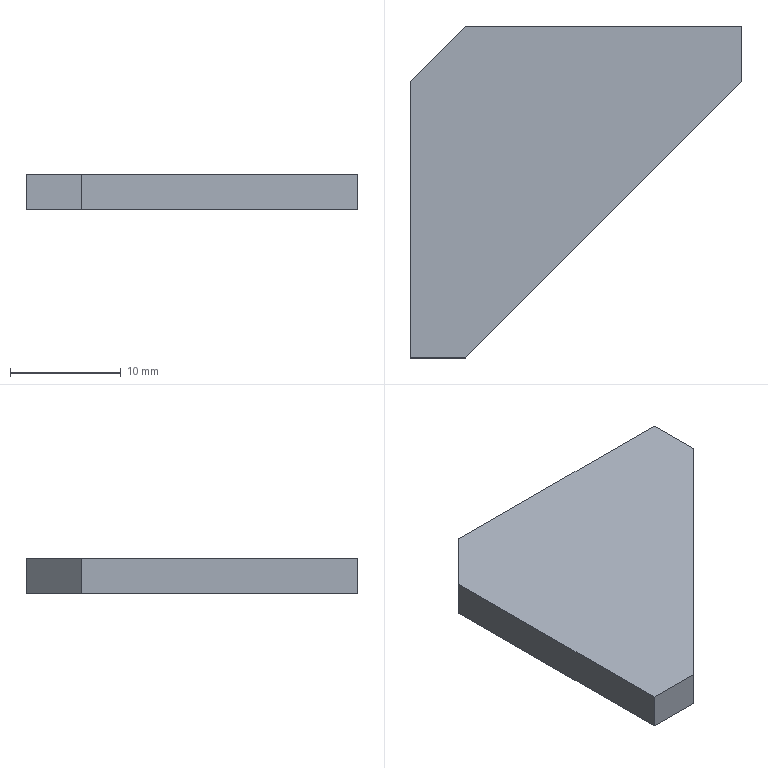Part | SolidWorks | features FlatPattern 1, SMBaseFlange 1, SheetMetal 1 | 1 solid | 8 faces | box 30 x 30 x 3.2 mm | volume 1840 mm3 | plane 8
STEP:
#1=CARTESIAN_POINT('',(268.2,-169.019,0.));
#2=VERTEX_POINT('',#1);
#3=CARTESIAN_POINT('',(243.2,-169.019,0.));
#4=VERTEX_POINT('',#3);
#5=CARTESIAN_POINT('',(243.2,-169.019,0.));
#6=DIRECTION('',(-1.,0.,0.));
#7=VECTOR('',#6,1000.);
#8=LINE('',#5,#7);
#9=EDGE_CURVE('',#2,#4,#8,.T.);
#10=ORIENTED_EDGE('',*,*,#9,.F.);
#11=CARTESIAN_POINT('',(268.2,-169.019,-3.2));
#12=VERTEX_POINT('',#11);
#13=CARTESIAN_POINT('',(268.2,-169.019,-3.2));
#14=DIRECTION('',(0.,0.,1.));
#15=VECTOR('',#14,1000.);
#16=LINE('',#13,#15);
#17=EDGE_CURVE('',#12,#2,#16,.T.);
#18=ORIENTED_EDGE('',*,*,#17,.F.);
#19=CARTESIAN_POINT('',(243.2,-169.019,-3.2));
#20=VERTEX_POINT('',#19);
#21=CARTESIAN_POINT('',(243.2,-169.019,-3.2));
#22=DIRECTION('',(-1.,0.,0.));
#23=VECTOR('',#22,1000.);
#24=LINE('',#21,#23);
#25=EDGE_CURVE('',#12,#20,#24,.T.);
#26=ORIENTED_EDGE('',*,*,#25,.T.);
#27=CARTESIAN_POINT('',(243.2,-169.019,-3.2));
#28=DIRECTION('',(0.,0.,1.));
#29=VECTOR('',#28,1000.);
#30=LINE('',#27,#29);
#31=EDGE_CURVE('',#20,#4,#30,.T.);
#32=ORIENTED_EDGE('',*,*,#31,.T.);
#33=EDGE_LOOP('',(#10,#18,#26,#32));
#34=FACE_OUTER_BOUND('',#33,.T.);
#35=CARTESIAN_POINT('',(243.2,-169.019,-3.2));
#36=DIRECTION('',(0.,1.,0.));
#37=DIRECTION('',(0.,0.,1.));
#38=AXIS2_PLACEMENT_3D('',#35,#36,#37);
#39=PLANE('',#38);
#40=ADVANCED_FACE('',(#34),#39,.T.);
#41=CARTESIAN_POINT('',(268.2,-174.019,0.));
#42=VERTEX_POINT('',#41);
#43=CARTESIAN_POINT('',(268.2,-169.019,0.));
#44=DIRECTION('',(0.,1.,0.));
#45=VECTOR('',#44,1000.);
#46=LINE('',#43,#45);
#47=EDGE_CURVE('',#42,#2,#46,.T.);
#48=ORIENTED_EDGE('',*,*,#47,.F.);
#49=CARTESIAN_POINT('',(268.2,-174.019,-3.2));
#50=VERTEX_POINT('',#49);
#51=CARTESIAN_POINT('',(268.2,-174.019,-3.2));
#52=DIRECTION('',(0.,0.,1.));
#53=VECTOR('',#52,1000.);
#54=LINE('',#51,#53);
#55=EDGE_CURVE('',#50,#42,#54,.T.);
#56=ORIENTED_EDGE('',*,*,#55,.F.);
#57=CARTESIAN_POINT('',(268.2,-169.019,-3.2));
#58=DIRECTION('',(0.,1.,0.));
#59=VECTOR('',#58,1000.);
#60=LINE('',#57,#59);
#61=EDGE_CURVE('',#50,#12,#60,.T.);
#62=ORIENTED_EDGE('',*,*,#61,.T.);
#63=ORIENTED_EDGE('',*,*,#17,.T.);
#64=EDGE_LOOP('',(#48,#56,#62,#63));
#65=FACE_OUTER_BOUND('',#64,.T.);
#66=CARTESIAN_POINT('',(268.2,-169.019,-3.2));
#67=DIRECTION('',(1.,0.,0.));
#68=DIRECTION('',(0.,0.,-1.));
#69=AXIS2_PLACEMENT_3D('',#66,#67,#68);
#70=PLANE('',#69);
#71=ADVANCED_FACE('',(#65),#70,.T.);
#72=CARTESIAN_POINT('',(243.2,-199.019,0.));
#73=VERTEX_POINT('',#72);
#74=CARTESIAN_POINT('',(268.2,-174.019,0.));
#75=DIRECTION('',(0.7071,0.7071,0.));
#76=VECTOR('',#75,1000.);
#77=LINE('',#74,#76);
#78=EDGE_CURVE('',#73,#42,#77,.T.);
#79=ORIENTED_EDGE('',*,*,#78,.F.);
#80=CARTESIAN_POINT('',(243.2,-199.019,-3.2));
#81=VERTEX_POINT('',#80);
#82=CARTESIAN_POINT('',(243.2,-199.019,-3.2));
#83=DIRECTION('',(0.,0.,1.));
#84=VECTOR('',#83,1000.);
#85=LINE('',#82,#84);
#86=EDGE_CURVE('',#81,#73,#85,.T.);
#87=ORIENTED_EDGE('',*,*,#86,.F.);
#88=CARTESIAN_POINT('',(268.2,-174.019,-3.2));
#89=DIRECTION('',(0.7071,0.7071,0.));
#90=VECTOR('',#89,1000.);
#91=LINE('',#88,#90);
#92=EDGE_CURVE('',#81,#50,#91,.T.);
#93=ORIENTED_EDGE('',*,*,#92,.T.);
#94=ORIENTED_EDGE('',*,*,#55,.T.);
#95=EDGE_LOOP('',(#79,#87,#93,#94));
#96=FACE_OUTER_BOUND('',#95,.T.);
#97=CARTESIAN_POINT('',(268.2,-174.019,-3.2));
#98=DIRECTION('',(0.7071,-0.7071,0.));
#99=DIRECTION('',(0.7071,0.7071,0.));
#100=AXIS2_PLACEMENT_3D('',#97,#98,#99);
#101=PLANE('',#100);
#102=ADVANCED_FACE('',(#96),#101,.T.);
#103=CARTESIAN_POINT('',(238.2,-199.019,0.));
#104=VERTEX_POINT('',#103);
#105=CARTESIAN_POINT('',(243.2,-199.019,0.));
#106=DIRECTION('',(1.,0.,0.));
#107=VECTOR('',#106,1000.);
#108=LINE('',#105,#107);
#109=EDGE_CURVE('',#104,#73,#108,.T.);
#110=ORIENTED_EDGE('',*,*,#109,.F.);
#111=CARTESIAN_POINT('',(238.2,-199.019,-3.2));
#112=VERTEX_POINT('',#111);
#113=CARTESIAN_POINT('',(238.2,-199.019,-3.2));
#114=DIRECTION('',(0.,0.,1.));
#115=VECTOR('',#114,1000.);
#116=LINE('',#113,#115);
#117=EDGE_CURVE('',#112,#104,#116,.T.);
#118=ORIENTED_EDGE('',*,*,#117,.F.);
#119=CARTESIAN_POINT('',(243.2,-199.019,-3.2));
#120=DIRECTION('',(1.,0.,0.));
#121=VECTOR('',#120,1000.);
#122=LINE('',#119,#121);
#123=EDGE_CURVE('',#112,#81,#122,.T.);
#124=ORIENTED_EDGE('',*,*,#123,.T.);
#125=ORIENTED_EDGE('',*,*,#86,.T.);
#126=EDGE_LOOP('',(#110,#118,#124,#125));
#127=FACE_OUTER_BOUND('',#126,.T.);
#128=CARTESIAN_POINT('',(243.2,-199.019,-3.2));
#129=DIRECTION('',(0.,-1.,0.));
#130=DIRECTION('',(0.,0.,-1.));
#131=AXIS2_PLACEMENT_3D('',#128,#129,#130);
#132=PLANE('',#131);
#133=ADVANCED_FACE('',(#127),#132,.T.);
#134=CARTESIAN_POINT('',(238.2,-174.019,0.));
#135=VERTEX_POINT('',#134);
#136=CARTESIAN_POINT('',(238.2,-199.019,0.));
#137=DIRECTION('',(0.,-1.,0.));
#138=VECTOR('',#137,1000.);
#139=LINE('',#136,#138);
#140=EDGE_CURVE('',#135,#104,#139,.T.);
#141=ORIENTED_EDGE('',*,*,#140,.F.);
#142=CARTESIAN_POINT('',(238.2,-174.019,-3.2));
#143=VERTEX_POINT('',#142);
#144=CARTESIAN_POINT('',(238.2,-174.019,-3.2));
#145=DIRECTION('',(0.,0.,1.));
#146=VECTOR('',#145,1000.);
#147=LINE('',#144,#146);
#148=EDGE_CURVE('',#143,#135,#147,.T.);
#149=ORIENTED_EDGE('',*,*,#148,.F.);
#150=CARTESIAN_POINT('',(238.2,-199.019,-3.2));
#151=DIRECTION('',(0.,-1.,0.));
#152=VECTOR('',#151,1000.);
#153=LINE('',#150,#152);
#154=EDGE_CURVE('',#143,#112,#153,.T.);
#155=ORIENTED_EDGE('',*,*,#154,.T.);
#156=ORIENTED_EDGE('',*,*,#117,.T.);
#157=EDGE_LOOP('',(#141,#149,#155,#156));
#158=FACE_OUTER_BOUND('',#157,.T.);
#159=CARTESIAN_POINT('',(238.2,-199.019,-3.2));
#160=DIRECTION('',(-1.,0.,0.));
#161=DIRECTION('',(0.,0.,1.));
#162=AXIS2_PLACEMENT_3D('',#159,#160,#161);
#163=PLANE('',#162);
#164=ADVANCED_FACE('',(#158),#163,.T.);
#165=CARTESIAN_POINT('',(238.2,-174.019,0.));
#166=DIRECTION('',(-0.7071,-0.7071,0.));
#167=VECTOR('',#166,1000.);
#168=LINE('',#165,#167);
#169=EDGE_CURVE('',#4,#135,#168,.T.);
#170=ORIENTED_EDGE('',*,*,#169,.F.);
#171=ORIENTED_EDGE('',*,*,#31,.F.);
#172=CARTESIAN_POINT('',(238.2,-174.019,-3.2));
#173=DIRECTION('',(-0.7071,-0.7071,0.));
#174=VECTOR('',#173,1000.);
#175=LINE('',#172,#174);
#176=EDGE_CURVE('',#20,#143,#175,.T.);
#177=ORIENTED_EDGE('',*,*,#176,.T.);
#178=ORIENTED_EDGE('',*,*,#148,.T.);
#179=EDGE_LOOP('',(#170,#171,#177,#178));
#180=FACE_OUTER_BOUND('',#179,.T.);
#181=CARTESIAN_POINT('',(238.2,-174.019,-3.2));
#182=DIRECTION('',(-0.7071,0.7071,0.));
#183=DIRECTION('',(-0.7071,-0.7071,0.));
#184=AXIS2_PLACEMENT_3D('',#181,#182,#183);
#185=PLANE('',#184);
#186=ADVANCED_FACE('',(#180),#185,.T.);
#187=ORIENTED_EDGE('',*,*,#25,.F.);
#188=ORIENTED_EDGE('',*,*,#61,.F.);
#189=ORIENTED_EDGE('',*,*,#92,.F.);
#190=ORIENTED_EDGE('',*,*,#123,.F.);
#191=ORIENTED_EDGE('',*,*,#154,.F.);
#192=ORIENTED_EDGE('',*,*,#176,.F.);
#193=EDGE_LOOP('',(#187,#188,#189,#190,#191,#192));
#194=FACE_OUTER_BOUND('',#193,.T.);
#195=CARTESIAN_POINT('',(0.,0.,-3.2));
#196=DIRECTION('',(0.,0.,-1.));
#197=DIRECTION('',(-1.,0.,0.));
#198=AXIS2_PLACEMENT_3D('',#195,#196,#197);
#199=PLANE('',#198);
#200=ADVANCED_FACE('',(#194),#199,.T.);
#201=ORIENTED_EDGE('',*,*,#9,.T.);
#202=ORIENTED_EDGE('',*,*,#169,.T.);
#203=ORIENTED_EDGE('',*,*,#140,.T.);
#204=ORIENTED_EDGE('',*,*,#109,.T.);
#205=ORIENTED_EDGE('',*,*,#78,.T.);
#206=ORIENTED_EDGE('',*,*,#47,.T.);
#207=EDGE_LOOP('',(#201,#202,#203,#204,#205,#206));
#208=FACE_OUTER_BOUND('',#207,.T.);
#209=CARTESIAN_POINT('',(0.,0.,0.));
#210=DIRECTION('',(0.,0.,-1.));
#211=DIRECTION('',(-1.,0.,0.));
#212=AXIS2_PLACEMENT_3D('',#209,#210,#211);
#213=PLANE('',#212);
#214=ADVANCED_FACE('',(#208),#213,.F.);
#215=CLOSED_SHELL('',(#40,#71,#102,#133,#164,#186,#200,#214));
#216=MANIFOLD_SOLID_BREP('',#215);
#217=CARTESIAN_POINT('',(0.,0.,0.));
#218=DIRECTION('',(0.,0.,1.));
#219=DIRECTION('',(1.,0.,0.));
#220=AXIS2_PLACEMENT_3D('',#217,#218,#219);
#221=(LENGTH_UNIT()NAMED_UNIT(*)SI_UNIT(.MILLI.,.METRE.));
#222=UNCERTAINTY_MEASURE_WITH_UNIT(LENGTH_MEASURE(0.00001),#221,'','');
#223=(NAMED_UNIT(*)PLANE_ANGLE_UNIT()SI_UNIT($,.RADIAN.));
#224=(NAMED_UNIT(*)SI_UNIT($,.STERADIAN.)SOLID_ANGLE_UNIT());
#225=(GEOMETRIC_REPRESENTATION_CONTEXT(3)GLOBAL_UNCERTAINTY_ASSIGNED_CONTEXT((#222))GLOBAL_UNIT_ASSIGNED_CONTEXT((#221,#223,#224))REPRESENTATION_CONTEXT('',''));
#226=ADVANCED_BREP_SHAPE_REPRESENTATION('',(#216,#220),#225);